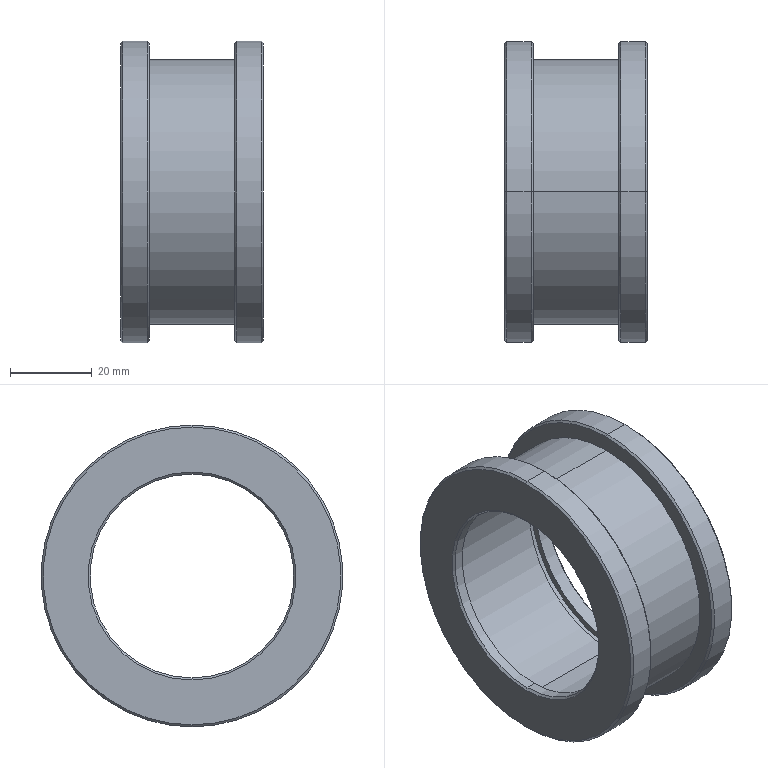Part | SolidWorks | features ICE 2, Chamfer 1, RevCut 1, Revolution 1 | 1 solid | 33 faces | box 35 x 74 x 74 mm | volume 47236 mm3 | cylinder 14 | cone 12 | plane 7 | commonest cylinder face diameters 55 x4 74 x4 50 x2 58 x2 65 x2
STEP:
#1=CARTESIAN_POINT('',(13.5,0.,-29.));
#2=VERTEX_POINT('',#1);
#3=CARTESIAN_POINT('',(13.5,0.,29.));
#4=VERTEX_POINT('',#3);
#5=CARTESIAN_POINT('',(13.5,0.,0.));
#6=DIRECTION('',(-1.,0.,0.));
#7=DIRECTION('',(0.,0.,1.));
#8=AXIS2_PLACEMENT_3D('',#5,#6,#7);
#9=CIRCLE('',#8,29.);
#10=EDGE_CURVE('',#2,#4,#9,.T.);
#11=ORIENTED_EDGE('',*,*,#10,.F.);
#12=CARTESIAN_POINT('',(11.3,0.,-29.));
#13=VERTEX_POINT('',#12);
#14=CARTESIAN_POINT('',(0.,0.,-29.));
#15=DIRECTION('',(-1.,0.,0.));
#16=VECTOR('',#15,1000.);
#17=LINE('',#14,#16);
#18=EDGE_CURVE('',#2,#13,#17,.T.);
#19=ORIENTED_EDGE('',*,*,#18,.T.);
#20=CARTESIAN_POINT('',(11.3,0.,29.));
#21=VERTEX_POINT('',#20);
#22=CARTESIAN_POINT('',(11.3,0.,0.));
#23=DIRECTION('',(-1.,0.,0.));
#24=DIRECTION('',(0.,0.,1.));
#25=AXIS2_PLACEMENT_3D('',#22,#23,#24);
#26=CIRCLE('',#25,29.);
#27=EDGE_CURVE('',#13,#21,#26,.T.);
#28=ORIENTED_EDGE('',*,*,#27,.T.);
#29=CARTESIAN_POINT('',(0.,0.,29.));
#30=DIRECTION('',(-1.,0.,0.));
#31=VECTOR('',#30,1000.);
#32=LINE('',#29,#31);
#33=EDGE_CURVE('',#4,#21,#32,.T.);
#34=ORIENTED_EDGE('',*,*,#33,.F.);
#35=EDGE_LOOP('',(#11,#19,#28,#34));
#36=FACE_OUTER_BOUND('',#35,.T.);
#37=CARTESIAN_POINT('',(0.,0.,0.));
#38=DIRECTION('',(-1.,0.,0.));
#39=DIRECTION('',(0.,0.,1.));
#40=AXIS2_PLACEMENT_3D('',#37,#38,#39);
#41=CYLINDRICAL_SURFACE('',#40,29.);
#42=ADVANCED_FACE('',(#36),#41,.F.);
#43=CARTESIAN_POINT('',(-10.5,0.,-36.5));
#44=VERTEX_POINT('',#43);
#45=CARTESIAN_POINT('',(-10.5,0.,36.5));
#46=VERTEX_POINT('',#45);
#47=CARTESIAN_POINT('',(-10.5,0.,0.));
#48=DIRECTION('',(1.,0.,0.));
#49=DIRECTION('',(0.,0.,1.));
#50=AXIS2_PLACEMENT_3D('',#47,#48,#49);
#51=CIRCLE('',#50,36.5);
#52=EDGE_CURVE('',#44,#46,#51,.T.);
#53=ORIENTED_EDGE('',*,*,#52,.F.);
#54=CARTESIAN_POINT('',(-11.,0.,-37.));
#55=VERTEX_POINT('',#54);
#56=CARTESIAN_POINT('',(-11.,0.,-37.));
#57=DIRECTION('',(-0.7071,0.,-0.7071));
#58=VECTOR('',#57,1000.);
#59=LINE('',#56,#58);
#60=EDGE_CURVE('',#44,#55,#59,.T.);
#61=ORIENTED_EDGE('',*,*,#60,.T.);
#62=CARTESIAN_POINT('',(-11.,0.,37.));
#63=VERTEX_POINT('',#62);
#64=CARTESIAN_POINT('',(-11.,0.,0.));
#65=DIRECTION('',(-1.,0.,0.));
#66=DIRECTION('',(0.,0.,1.));
#67=AXIS2_PLACEMENT_3D('',#64,#65,#66);
#68=CIRCLE('',#67,37.);
#69=EDGE_CURVE('',#63,#55,#68,.T.);
#70=ORIENTED_EDGE('',*,*,#69,.F.);
#71=CARTESIAN_POINT('',(-11.,0.,37.));
#72=DIRECTION('',(-0.7071,0.,0.7071));
#73=VECTOR('',#72,1000.);
#74=LINE('',#71,#73);
#75=EDGE_CURVE('',#46,#63,#74,.T.);
#76=ORIENTED_EDGE('',*,*,#75,.F.);
#77=EDGE_LOOP('',(#53,#61,#70,#76));
#78=FACE_OUTER_BOUND('',#77,.T.);
#79=CARTESIAN_POINT('',(-11.,0.,0.));
#80=DIRECTION('',(-1.,0.,0.));
#81=DIRECTION('',(0.,0.,1.));
#82=AXIS2_PLACEMENT_3D('',#79,#80,#81);
#83=CONICAL_SURFACE('',#82,37.,0.7854);
#84=ADVANCED_FACE('',(#78),#83,.T.);
#85=CARTESIAN_POINT('',(10.5,0.,36.5));
#86=VERTEX_POINT('',#85);
#87=CARTESIAN_POINT('',(10.5,0.,-36.5));
#88=VERTEX_POINT('',#87);
#89=CARTESIAN_POINT('',(10.5,0.,0.));
#90=DIRECTION('',(-1.,0.,0.));
#91=DIRECTION('',(0.,0.,-1.));
#92=AXIS2_PLACEMENT_3D('',#89,#90,#91);
#93=CIRCLE('',#92,36.5);
#94=EDGE_CURVE('',#86,#88,#93,.T.);
#95=ORIENTED_EDGE('',*,*,#94,.F.);
#96=CARTESIAN_POINT('',(11.,0.,37.));
#97=VERTEX_POINT('',#96);
#98=CARTESIAN_POINT('',(10.5,0.,36.5));
#99=DIRECTION('',(0.7071,0.,0.7071));
#100=VECTOR('',#99,1000.);
#101=LINE('',#98,#100);
#102=EDGE_CURVE('',#86,#97,#101,.T.);
#103=ORIENTED_EDGE('',*,*,#102,.T.);
#104=CARTESIAN_POINT('',(11.,0.,-37.));
#105=VERTEX_POINT('',#104);
#106=CARTESIAN_POINT('',(11.,0.,0.));
#107=DIRECTION('',(1.,0.,0.));
#108=DIRECTION('',(0.,0.,-1.));
#109=AXIS2_PLACEMENT_3D('',#106,#107,#108);
#110=CIRCLE('',#109,37.);
#111=EDGE_CURVE('',#105,#97,#110,.T.);
#112=ORIENTED_EDGE('',*,*,#111,.F.);
#113=CARTESIAN_POINT('',(10.5,0.,-36.5));
#114=DIRECTION('',(0.7071,0.,-0.7071));
#115=VECTOR('',#114,1000.);
#116=LINE('',#113,#115);
#117=EDGE_CURVE('',#88,#105,#116,.T.);
#118=ORIENTED_EDGE('',*,*,#117,.F.);
#119=EDGE_LOOP('',(#95,#103,#112,#118));
#120=FACE_OUTER_BOUND('',#119,.T.);
#121=CARTESIAN_POINT('',(10.5,0.,0.));
#122=DIRECTION('',(1.,0.,0.));
#123=DIRECTION('',(0.,0.,-1.));
#124=AXIS2_PLACEMENT_3D('',#121,#122,#123);
#125=CONICAL_SURFACE('',#124,36.5,0.7854);
#126=ADVANCED_FACE('',(#120),#125,.T.);
#127=CARTESIAN_POINT('',(17.5,0.,-36.5));
#128=VERTEX_POINT('',#127);
#129=CARTESIAN_POINT('',(17.5,0.,36.5));
#130=VERTEX_POINT('',#129);
#131=CARTESIAN_POINT('',(17.5,0.,0.));
#132=DIRECTION('',(1.,0.,0.));
#133=DIRECTION('',(0.,0.,1.));
#134=AXIS2_PLACEMENT_3D('',#131,#132,#133);
#135=CIRCLE('',#134,36.5);
#136=EDGE_CURVE('',#128,#130,#135,.T.);
#137=ORIENTED_EDGE('',*,*,#136,.F.);
#138=CARTESIAN_POINT('',(17.,0.,-37.));
#139=VERTEX_POINT('',#138);
#140=CARTESIAN_POINT('',(17.,0.,-37.));
#141=DIRECTION('',(-0.7071,0.,-0.7071));
#142=VECTOR('',#141,1000.);
#143=LINE('',#140,#142);
#144=EDGE_CURVE('',#128,#139,#143,.T.);
#145=ORIENTED_EDGE('',*,*,#144,.T.);
#146=CARTESIAN_POINT('',(17.,0.,37.));
#147=VERTEX_POINT('',#146);
#148=CARTESIAN_POINT('',(17.,0.,0.));
#149=DIRECTION('',(-1.,0.,0.));
#150=DIRECTION('',(0.,0.,1.));
#151=AXIS2_PLACEMENT_3D('',#148,#149,#150);
#152=CIRCLE('',#151,37.);
#153=EDGE_CURVE('',#147,#139,#152,.T.);
#154=ORIENTED_EDGE('',*,*,#153,.F.);
#155=CARTESIAN_POINT('',(17.,0.,37.));
#156=DIRECTION('',(-0.7071,0.,0.7071));
#157=VECTOR('',#156,1000.);
#158=LINE('',#155,#157);
#159=EDGE_CURVE('',#130,#147,#158,.T.);
#160=ORIENTED_EDGE('',*,*,#159,.F.);
#161=EDGE_LOOP('',(#137,#145,#154,#160));
#162=FACE_OUTER_BOUND('',#161,.T.);
#163=CARTESIAN_POINT('',(17.,0.,0.));
#164=DIRECTION('',(-1.,0.,0.));
#165=DIRECTION('',(0.,0.,1.));
#166=AXIS2_PLACEMENT_3D('',#163,#164,#165);
#167=CONICAL_SURFACE('',#166,37.,0.7854);
#168=ADVANCED_FACE('',(#162),#167,.T.);
#169=CARTESIAN_POINT('',(-17.5,0.,36.5));
#170=VERTEX_POINT('',#169);
#171=CARTESIAN_POINT('',(-17.5,0.,-36.5));
#172=VERTEX_POINT('',#171);
#173=CARTESIAN_POINT('',(-17.5,0.,0.));
#174=DIRECTION('',(-1.,0.,0.));
#175=DIRECTION('',(0.,0.,-1.));
#176=AXIS2_PLACEMENT_3D('',#173,#174,#175);
#177=CIRCLE('',#176,36.5);
#178=EDGE_CURVE('',#170,#172,#177,.T.);
#179=ORIENTED_EDGE('',*,*,#178,.F.);
#180=CARTESIAN_POINT('',(-17.,0.,37.));
#181=VERTEX_POINT('',#180);
#182=CARTESIAN_POINT('',(-17.5,0.,36.5));
#183=DIRECTION('',(0.7071,0.,0.7071));
#184=VECTOR('',#183,1000.);
#185=LINE('',#182,#184);
#186=EDGE_CURVE('',#170,#181,#185,.T.);
#187=ORIENTED_EDGE('',*,*,#186,.T.);
#188=CARTESIAN_POINT('',(-17.,0.,-37.));
#189=VERTEX_POINT('',#188);
#190=CARTESIAN_POINT('',(-17.,0.,0.));
#191=DIRECTION('',(1.,0.,0.));
#192=DIRECTION('',(0.,0.,-1.));
#193=AXIS2_PLACEMENT_3D('',#190,#191,#192);
#194=CIRCLE('',#193,37.);
#195=EDGE_CURVE('',#189,#181,#194,.T.);
#196=ORIENTED_EDGE('',*,*,#195,.F.);
#197=CARTESIAN_POINT('',(-17.5,0.,-36.5));
#198=DIRECTION('',(0.7071,0.,-0.7071));
#199=VECTOR('',#198,1000.);
#200=LINE('',#197,#199);
#201=EDGE_CURVE('',#172,#189,#200,.T.);
#202=ORIENTED_EDGE('',*,*,#201,.F.);
#203=EDGE_LOOP('',(#179,#187,#196,#202));
#204=FACE_OUTER_BOUND('',#203,.T.);
#205=CARTESIAN_POINT('',(-17.5,0.,0.));
#206=DIRECTION('',(1.,0.,0.));
#207=DIRECTION('',(0.,0.,-1.));
#208=AXIS2_PLACEMENT_3D('',#205,#206,#207);
#209=CONICAL_SURFACE('',#208,36.5,0.7854);
#210=ADVANCED_FACE('',(#204),#209,.T.);
#211=CARTESIAN_POINT('',(17.,0.,27.5));
#212=VERTEX_POINT('',#211);
#213=CARTESIAN_POINT('',(17.,0.,-27.5));
#214=VERTEX_POINT('',#213);
#215=CARTESIAN_POINT('',(17.,0.,0.));
#216=DIRECTION('',(1.,0.,0.));
#217=DIRECTION('',(0.,0.,1.));
#218=AXIS2_PLACEMENT_3D('',#215,#216,#217);
#219=CIRCLE('',#218,27.5);
#220=EDGE_CURVE('',#212,#214,#219,.T.);
#221=ORIENTED_EDGE('',*,*,#220,.F.);
#222=CARTESIAN_POINT('',(17.5,0.,28.));
#223=VERTEX_POINT('',#222);
#224=CARTESIAN_POINT('',(17.,0.,27.5));
#225=DIRECTION('',(0.7071,0.,0.7071));
#226=VECTOR('',#225,1000.);
#227=LINE('',#224,#226);
#228=EDGE_CURVE('',#212,#223,#227,.T.);
#229=ORIENTED_EDGE('',*,*,#228,.T.);
#230=CARTESIAN_POINT('',(17.5,0.,-28.));
#231=VERTEX_POINT('',#230);
#232=CARTESIAN_POINT('',(17.5,0.,0.));
#233=DIRECTION('',(-1.,0.,0.));
#234=DIRECTION('',(0.,0.,1.));
#235=AXIS2_PLACEMENT_3D('',#232,#233,#234);
#236=CIRCLE('',#235,28.);
#237=EDGE_CURVE('',#231,#223,#236,.T.);
#238=ORIENTED_EDGE('',*,*,#237,.F.);
#239=CARTESIAN_POINT('',(17.,0.,-27.5));
#240=DIRECTION('',(0.7071,0.,-0.7071));
#241=VECTOR('',#240,1000.);
#242=LINE('',#239,#241);
#243=EDGE_CURVE('',#214,#231,#242,.T.);
#244=ORIENTED_EDGE('',*,*,#243,.F.);
#245=EDGE_LOOP('',(#221,#229,#238,#244));
#246=FACE_OUTER_BOUND('',#245,.T.);
#247=CARTESIAN_POINT('',(17.,0.,0.));
#248=DIRECTION('',(1.,0.,0.));
#249=DIRECTION('',(0.,0.,-1.));
#250=AXIS2_PLACEMENT_3D('',#247,#248,#249);
#251=CONICAL_SURFACE('',#250,27.5,0.7854);
#252=ADVANCED_FACE('',(#246),#251,.F.);
#253=CARTESIAN_POINT('',(-17.,0.,-25.));
#254=VERTEX_POINT('',#253);
#255=CARTESIAN_POINT('',(-17.,0.,25.));
#256=VERTEX_POINT('',#255);
#257=CARTESIAN_POINT('',(-17.,0.,0.));
#258=DIRECTION('',(-1.,0.,0.));
#259=DIRECTION('',(0.,0.,-1.));
#260=AXIS2_PLACEMENT_3D('',#257,#258,#259);
#261=CIRCLE('',#260,25.);
#262=EDGE_CURVE('',#254,#256,#261,.T.);
#263=ORIENTED_EDGE('',*,*,#262,.F.);
#264=CARTESIAN_POINT('',(-17.5,0.,-25.5));
#265=VERTEX_POINT('',#264);
#266=CARTESIAN_POINT('',(-17.5,0.,-25.5));
#267=DIRECTION('',(-0.7071,0.,-0.7071));
#268=VECTOR('',#267,1000.);
#269=LINE('',#266,#268);
#270=EDGE_CURVE('',#254,#265,#269,.T.);
#271=ORIENTED_EDGE('',*,*,#270,.T.);
#272=CARTESIAN_POINT('',(-17.5,0.,25.5));
#273=VERTEX_POINT('',#272);
#274=CARTESIAN_POINT('',(-17.5,0.,0.));
#275=DIRECTION('',(1.,0.,0.));
#276=DIRECTION('',(0.,0.,-1.));
#277=AXIS2_PLACEMENT_3D('',#274,#275,#276);
#278=CIRCLE('',#277,25.5);
#279=EDGE_CURVE('',#273,#265,#278,.T.);
#280=ORIENTED_EDGE('',*,*,#279,.F.);
#281=CARTESIAN_POINT('',(-17.5,0.,25.5));
#282=DIRECTION('',(-0.7071,0.,0.7071));
#283=VECTOR('',#282,1000.);
#284=LINE('',#281,#283);
#285=EDGE_CURVE('',#256,#273,#284,.T.);
#286=ORIENTED_EDGE('',*,*,#285,.F.);
#287=EDGE_LOOP('',(#263,#271,#280,#286));
#288=FACE_OUTER_BOUND('',#287,.T.);
#289=CARTESIAN_POINT('',(-17.5,0.,0.));
#290=DIRECTION('',(-1.,0.,0.));
#291=DIRECTION('',(0.,0.,1.));
#292=AXIS2_PLACEMENT_3D('',#289,#290,#291);
#293=CONICAL_SURFACE('',#292,25.5,0.7854);
#294=ADVANCED_FACE('',(#288),#293,.F.);
#295=ORIENTED_EDGE('',*,*,#262,.T.);
#296=CARTESIAN_POINT('',(-14.5,0.,25.));
#297=VERTEX_POINT('',#296);
#298=CARTESIAN_POINT('',(-44.5,0.,25.));
#299=DIRECTION('',(1.,0.,0.));
#300=VECTOR('',#299,1000.);
#301=LINE('',#298,#300);
#302=EDGE_CURVE('',#256,#297,#301,.T.);
#303=ORIENTED_EDGE('',*,*,#302,.T.);
#304=CARTESIAN_POINT('',(-14.5,0.,-25.));
#305=VERTEX_POINT('',#304);
#306=CARTESIAN_POINT('',(-14.5,0.,0.));
#307=DIRECTION('',(1.,0.,0.));
#308=DIRECTION('',(0.,0.,-1.));
#309=AXIS2_PLACEMENT_3D('',#306,#307,#308);
#310=CIRCLE('',#309,25.);
#311=EDGE_CURVE('',#297,#305,#310,.T.);
#312=ORIENTED_EDGE('',*,*,#311,.T.);
#313=CARTESIAN_POINT('',(-44.5,0.,-25.));
#314=DIRECTION('',(1.,0.,0.));
#315=VECTOR('',#314,1000.);
#316=LINE('',#313,#315);
#317=EDGE_CURVE('',#254,#305,#316,.T.);
#318=ORIENTED_EDGE('',*,*,#317,.F.);
#319=EDGE_LOOP('',(#295,#303,#312,#318));
#320=FACE_OUTER_BOUND('',#319,.T.);
#321=CARTESIAN_POINT('',(-44.5,0.,0.));
#322=DIRECTION('',(1.,0.,0.));
#323=DIRECTION('',(0.,0.,-1.));
#324=AXIS2_PLACEMENT_3D('',#321,#322,#323);
#325=CYLINDRICAL_SURFACE('',#324,25.);
#326=ADVANCED_FACE('',(#320),#325,.F.);
#327=ORIENTED_EDGE('',*,*,#69,.T.);
#328=CARTESIAN_POINT('',(-17.5,0.,-37.));
#329=DIRECTION('',(-1.,0.,0.));
#330=VECTOR('',#329,1000.);
#331=LINE('',#328,#330);
#332=EDGE_CURVE('',#55,#189,#331,.T.);
#333=ORIENTED_EDGE('',*,*,#332,.T.);
#334=ORIENTED_EDGE('',*,*,#195,.T.);
#335=CARTESIAN_POINT('',(-17.5,0.,37.));
#336=DIRECTION('',(-1.,0.,0.));
#337=VECTOR('',#336,1000.);
#338=LINE('',#335,#337);
#339=EDGE_CURVE('',#63,#181,#338,.T.);
#340=ORIENTED_EDGE('',*,*,#339,.F.);
#341=EDGE_LOOP('',(#327,#333,#334,#340));
#342=FACE_OUTER_BOUND('',#341,.T.);
#343=CARTESIAN_POINT('',(-17.5,0.,0.));
#344=DIRECTION('',(-1.,0.,0.));
#345=DIRECTION('',(0.,0.,1.));
#346=AXIS2_PLACEMENT_3D('',#343,#344,#345);
#347=CYLINDRICAL_SURFACE('',#346,37.);
#348=ADVANCED_FACE('',(#342),#347,.T.);
#349=CARTESIAN_POINT('',(10.5,0.,32.5));
#350=VERTEX_POINT('',#349);
#351=CARTESIAN_POINT('',(10.5,0.,-32.5));
#352=VERTEX_POINT('',#351);
#353=CARTESIAN_POINT('',(10.5,0.,0.));
#354=DIRECTION('',(-1.,0.,0.));
#355=DIRECTION('',(0.,0.,1.));
#356=AXIS2_PLACEMENT_3D('',#353,#354,#355);
#357=CIRCLE('',#356,32.5);
#358=EDGE_CURVE('',#350,#352,#357,.T.);
#359=ORIENTED_EDGE('',*,*,#358,.T.);
#360=CARTESIAN_POINT('',(-10.5,0.,-32.5));
#361=VERTEX_POINT('',#360);
#362=CARTESIAN_POINT('',(-17.5,0.,-32.5));
#363=DIRECTION('',(-1.,0.,0.));
#364=VECTOR('',#363,1000.);
#365=LINE('',#362,#364);
#366=EDGE_CURVE('',#352,#361,#365,.T.);
#367=ORIENTED_EDGE('',*,*,#366,.T.);
#368=CARTESIAN_POINT('',(-10.5,0.,32.5));
#369=VERTEX_POINT('',#368);
#370=CARTESIAN_POINT('',(-10.5,0.,0.));
#371=DIRECTION('',(-1.,0.,0.));
#372=DIRECTION('',(0.,0.,1.));
#373=AXIS2_PLACEMENT_3D('',#370,#371,#372);
#374=CIRCLE('',#373,32.5);
#375=EDGE_CURVE('',#369,#361,#374,.T.);
#376=ORIENTED_EDGE('',*,*,#375,.F.);
#377=CARTESIAN_POINT('',(-17.5,0.,32.5));
#378=DIRECTION('',(-1.,0.,0.));
#379=VECTOR('',#378,1000.);
#380=LINE('',#377,#379);
#381=EDGE_CURVE('',#350,#369,#380,.T.);
#382=ORIENTED_EDGE('',*,*,#381,.F.);
#383=EDGE_LOOP('',(#359,#367,#376,#382));
#384=FACE_OUTER_BOUND('',#383,.T.);
#385=CARTESIAN_POINT('',(-17.5,0.,0.));
#386=DIRECTION('',(-1.,0.,0.));
#387=DIRECTION('',(0.,0.,1.));
#388=AXIS2_PLACEMENT_3D('',#385,#386,#387);
#389=CYLINDRICAL_SURFACE('',#388,32.5);
#390=ADVANCED_FACE('',(#384),#389,.T.);
#391=ORIENTED_EDGE('',*,*,#153,.T.);
#392=CARTESIAN_POINT('',(-17.5,0.,-37.));
#393=DIRECTION('',(-1.,0.,0.));
#394=VECTOR('',#393,1000.);
#395=LINE('',#392,#394);
#396=EDGE_CURVE('',#139,#105,#395,.T.);
#397=ORIENTED_EDGE('',*,*,#396,.T.);
#398=ORIENTED_EDGE('',*,*,#111,.T.);
#399=CARTESIAN_POINT('',(-17.5,0.,37.));
#400=DIRECTION('',(-1.,0.,0.));
#401=VECTOR('',#400,1000.);
#402=LINE('',#399,#401);
#403=EDGE_CURVE('',#147,#97,#402,.T.);
#404=ORIENTED_EDGE('',*,*,#403,.F.);
#405=EDGE_LOOP('',(#391,#397,#398,#404));
#406=FACE_OUTER_BOUND('',#405,.T.);
#407=CARTESIAN_POINT('',(-17.5,0.,0.));
#408=DIRECTION('',(-1.,0.,0.));
#409=DIRECTION('',(0.,0.,1.));
#410=AXIS2_PLACEMENT_3D('',#407,#408,#409);
#411=CYLINDRICAL_SURFACE('',#410,37.);
#412=ADVANCED_FACE('',(#406),#411,.T.);
#413=CARTESIAN_POINT('',(13.5,0.,-27.5));
#414=VERTEX_POINT('',#413);
#415=CARTESIAN_POINT('',(13.5,0.,27.5));
#416=VERTEX_POINT('',#415);
#417=CARTESIAN_POINT('',(13.5,0.,0.));
#418=DIRECTION('',(-1.,0.,0.));
#419=DIRECTION('',(0.,0.,1.));
#420=AXIS2_PLACEMENT_3D('',#417,#418,#419);
#421=CIRCLE('',#420,27.5);
#422=EDGE_CURVE('',#414,#416,#421,.T.);
#423=ORIENTED_EDGE('',*,*,#422,.T.);
#424=CARTESIAN_POINT('',(-14.5,0.,27.5));
#425=DIRECTION('',(1.,0.,0.));
#426=VECTOR('',#425,1000.);
#427=LINE('',#424,#426);
#428=EDGE_CURVE('',#416,#212,#427,.T.);
#429=ORIENTED_EDGE('',*,*,#428,.T.);
#430=ORIENTED_EDGE('',*,*,#220,.T.);
#431=CARTESIAN_POINT('',(-14.5,0.,-27.5));
#432=DIRECTION('',(1.,0.,0.));
#433=VECTOR('',#432,1000.);
#434=LINE('',#431,#433);
#435=EDGE_CURVE('',#414,#214,#434,.T.);
#436=ORIENTED_EDGE('',*,*,#435,.F.);
#437=EDGE_LOOP('',(#423,#429,#430,#436));
#438=FACE_OUTER_BOUND('',#437,.T.);
#439=CARTESIAN_POINT('',(-14.5,0.,0.));
#440=DIRECTION('',(1.,0.,0.));
#441=DIRECTION('',(0.,0.,-1.));
#442=AXIS2_PLACEMENT_3D('',#439,#440,#441);
#443=CYLINDRICAL_SURFACE('',#442,27.5);
#444=ADVANCED_FACE('',(#438),#443,.F.);
#445=CARTESIAN_POINT('',(-14.5,0.,27.5));
#446=VERTEX_POINT('',#445);
#447=CARTESIAN_POINT('',(-14.5,0.,-27.5));
#448=VERTEX_POINT('',#447);
#449=CARTESIAN_POINT('',(-14.5,0.,0.));
#450=DIRECTION('',(1.,0.,0.));
#451=DIRECTION('',(0.,0.,-1.));
#452=AXIS2_PLACEMENT_3D('',#449,#450,#451);
#453=CIRCLE('',#452,27.5);
#454=EDGE_CURVE('',#446,#448,#453,.T.);
#455=ORIENTED_EDGE('',*,*,#454,.F.);
#456=CARTESIAN_POINT('',(11.3,0.,27.5));
#457=VERTEX_POINT('',#456);
#458=CARTESIAN_POINT('',(-14.5,0.,27.5));
#459=DIRECTION('',(1.,0.,0.));
#460=VECTOR('',#459,1000.);
#461=LINE('',#458,#460);
#462=EDGE_CURVE('',#446,#457,#461,.T.);
#463=ORIENTED_EDGE('',*,*,#462,.T.);
#464=CARTESIAN_POINT('',(11.3,0.,-27.5));
#465=VERTEX_POINT('',#464);
#466=CARTESIAN_POINT('',(11.3,0.,0.));
#467=DIRECTION('',(-1.,0.,0.));
#468=DIRECTION('',(0.,0.,1.));
#469=AXIS2_PLACEMENT_3D('',#466,#467,#468);
#470=CIRCLE('',#469,27.5);
#471=EDGE_CURVE('',#465,#457,#470,.T.);
#472=ORIENTED_EDGE('',*,*,#471,.F.);
#473=CARTESIAN_POINT('',(-14.5,0.,-27.5));
#474=DIRECTION('',(1.,0.,0.));
#475=VECTOR('',#474,1000.);
#476=LINE('',#473,#475);
#477=EDGE_CURVE('',#448,#465,#476,.T.);
#478=ORIENTED_EDGE('',*,*,#477,.F.);
#479=EDGE_LOOP('',(#455,#463,#472,#478));
#480=FACE_OUTER_BOUND('',#479,.T.);
#481=CARTESIAN_POINT('',(-14.5,0.,0.));
#482=DIRECTION('',(1.,0.,0.));
#483=DIRECTION('',(0.,0.,-1.));
#484=AXIS2_PLACEMENT_3D('',#481,#482,#483);
#485=CYLINDRICAL_SURFACE('',#484,27.5);
#486=ADVANCED_FACE('',(#480),#485,.F.);
#487=ORIENTED_EDGE('',*,*,#462,.F.);
#488=CARTESIAN_POINT('',(-14.5,0.,0.));
#489=DIRECTION('',(1.,0.,0.));
#490=DIRECTION('',(0.,0.,-1.));
#491=AXIS2_PLACEMENT_3D('',#488,#489,#490);
#492=CIRCLE('',#491,27.5);
#493=EDGE_CURVE('',#448,#446,#492,.T.);
#494=ORIENTED_EDGE('',*,*,#493,.F.);
#495=ORIENTED_EDGE('',*,*,#477,.T.);
#496=CARTESIAN_POINT('',(11.3,0.,0.));
#497=DIRECTION('',(-1.,0.,0.));
#498=DIRECTION('',(0.,0.,1.));
#499=AXIS2_PLACEMENT_3D('',#496,#497,#498);
#500=CIRCLE('',#499,27.5);
#501=EDGE_CURVE('',#457,#465,#500,.T.);
#502=ORIENTED_EDGE('',*,*,#501,.F.);
#503=EDGE_LOOP('',(#487,#494,#495,#502));
#504=FACE_OUTER_BOUND('',#503,.T.);
#505=CARTESIAN_POINT('',(-14.5,0.,0.));
#506=DIRECTION('',(1.,0.,0.));
#507=DIRECTION('',(0.,0.,-1.));
#508=AXIS2_PLACEMENT_3D('',#505,#506,#507);
#509=CYLINDRICAL_SURFACE('',#508,27.5);
#510=ADVANCED_FACE('',(#504),#509,.F.);
#511=ORIENTED_EDGE('',*,*,#428,.F.);
#512=CARTESIAN_POINT('',(13.5,0.,0.));
#513=DIRECTION('',(-1.,0.,0.));
#514=DIRECTION('',(0.,0.,1.));
#515=AXIS2_PLACEMENT_3D('',#512,#513,#514);
#516=CIRCLE('',#515,27.5);
#517=EDGE_CURVE('',#416,#414,#516,.T.);
#518=ORIENTED_EDGE('',*,*,#517,.T.);
#519=ORIENTED_EDGE('',*,*,#435,.T.);
#520=CARTESIAN_POINT('',(17.,0.,0.));
#521=DIRECTION('',(1.,0.,0.));
#522=DIRECTION('',(0.,0.,1.));
#523=AXIS2_PLACEMENT_3D('',#520,#521,#522);
#524=CIRCLE('',#523,27.5);
#525=EDGE_CURVE('',#214,#212,#524,.T.);
#526=ORIENTED_EDGE('',*,*,#525,.T.);
#527=EDGE_LOOP('',(#511,#518,#519,#526));
#528=FACE_OUTER_BOUND('',#527,.T.);
#529=CARTESIAN_POINT('',(-14.5,0.,0.));
#530=DIRECTION('',(1.,0.,0.));
#531=DIRECTION('',(0.,0.,-1.));
#532=AXIS2_PLACEMENT_3D('',#529,#530,#531);
#533=CYLINDRICAL_SURFACE('',#532,27.5);
#534=ADVANCED_FACE('',(#528),#533,.F.);
#535=ORIENTED_EDGE('',*,*,#279,.T.);
#536=CARTESIAN_POINT('',(-17.5,0.,0.));
#537=DIRECTION('',(1.,0.,0.));
#538=DIRECTION('',(0.,0.,-1.));
#539=AXIS2_PLACEMENT_3D('',#536,#537,#538);
#540=CIRCLE('',#539,25.5);
#541=EDGE_CURVE('',#265,#273,#540,.T.);
#542=ORIENTED_EDGE('',*,*,#541,.T.);
#543=EDGE_LOOP('',(#535,#542));
#544=FACE_BOUND('',#543,.T.);
#545=CARTESIAN_POINT('',(-17.5,0.,0.));
#546=DIRECTION('',(-1.,0.,0.));
#547=DIRECTION('',(0.,0.,-1.));
#548=AXIS2_PLACEMENT_3D('',#545,#546,#547);
#549=CIRCLE('',#548,36.5);
#550=EDGE_CURVE('',#172,#170,#549,.T.);
#551=ORIENTED_EDGE('',*,*,#550,.T.);
#552=ORIENTED_EDGE('',*,*,#178,.T.);
#553=EDGE_LOOP('',(#551,#552));
#554=FACE_OUTER_BOUND('',#553,.T.);
#555=CARTESIAN_POINT('',(-17.5,37.,0.));
#556=DIRECTION('',(1.,0.,0.));
#557=DIRECTION('',(0.,0.,-1.));
#558=AXIS2_PLACEMENT_3D('',#555,#556,#557);
#559=PLANE('',#558);
#560=ADVANCED_FACE('',(#544,#554),#559,.F.);
#561=ORIENTED_EDGE('',*,*,#237,.T.);
#562=CARTESIAN_POINT('',(17.5,0.,0.));
#563=DIRECTION('',(-1.,0.,0.));
#564=DIRECTION('',(0.,0.,1.));
#565=AXIS2_PLACEMENT_3D('',#562,#563,#564);
#566=CIRCLE('',#565,28.);
#567=EDGE_CURVE('',#223,#231,#566,.T.);
#568=ORIENTED_EDGE('',*,*,#567,.T.);
#569=EDGE_LOOP('',(#561,#568));
#570=FACE_BOUND('',#569,.T.);
#571=CARTESIAN_POINT('',(17.5,0.,0.));
#572=DIRECTION('',(1.,0.,0.));
#573=DIRECTION('',(0.,0.,1.));
#574=AXIS2_PLACEMENT_3D('',#571,#572,#573);
#575=CIRCLE('',#574,36.5);
#576=EDGE_CURVE('',#130,#128,#575,.T.);
#577=ORIENTED_EDGE('',*,*,#576,.T.);
#578=ORIENTED_EDGE('',*,*,#136,.T.);
#579=EDGE_LOOP('',(#577,#578));
#580=FACE_OUTER_BOUND('',#579,.T.);
#581=CARTESIAN_POINT('',(17.5,0.,0.));
#582=DIRECTION('',(-1.,0.,0.));
#583=DIRECTION('',(0.,0.,1.));
#584=AXIS2_PLACEMENT_3D('',#581,#582,#583);
#585=PLANE('',#584);
#586=ADVANCED_FACE('',(#570,#580),#585,.F.);
#587=ORIENTED_EDGE('',*,*,#396,.F.);
#588=CARTESIAN_POINT('',(17.,0.,0.));
#589=DIRECTION('',(-1.,0.,0.));
#590=DIRECTION('',(0.,0.,1.));
#591=AXIS2_PLACEMENT_3D('',#588,#589,#590);
#592=CIRCLE('',#591,37.);
#593=EDGE_CURVE('',#139,#147,#592,.T.);
#594=ORIENTED_EDGE('',*,*,#593,.T.);
#595=ORIENTED_EDGE('',*,*,#403,.T.);
#596=CARTESIAN_POINT('',(11.,0.,0.));
#597=DIRECTION('',(1.,0.,0.));
#598=DIRECTION('',(0.,0.,-1.));
#599=AXIS2_PLACEMENT_3D('',#596,#597,#598);
#600=CIRCLE('',#599,37.);
#601=EDGE_CURVE('',#97,#105,#600,.T.);
#602=ORIENTED_EDGE('',*,*,#601,.T.);
#603=EDGE_LOOP('',(#587,#594,#595,#602));
#604=FACE_OUTER_BOUND('',#603,.T.);
#605=CARTESIAN_POINT('',(-17.5,0.,0.));
#606=DIRECTION('',(-1.,0.,0.));
#607=DIRECTION('',(0.,0.,1.));
#608=AXIS2_PLACEMENT_3D('',#605,#606,#607);
#609=CYLINDRICAL_SURFACE('',#608,37.);
#610=ADVANCED_FACE('',(#604),#609,.T.);
#611=CARTESIAN_POINT('',(10.5,0.,0.));
#612=DIRECTION('',(-1.,0.,0.));
#613=DIRECTION('',(0.,0.,-1.));
#614=AXIS2_PLACEMENT_3D('',#611,#612,#613);
#615=CIRCLE('',#614,36.5);
#616=EDGE_CURVE('',#88,#86,#615,.T.);
#617=ORIENTED_EDGE('',*,*,#616,.T.);
#618=ORIENTED_EDGE('',*,*,#94,.T.);
#619=EDGE_LOOP('',(#617,#618));
#620=FACE_OUTER_BOUND('',#619,.T.);
#621=ORIENTED_EDGE('',*,*,#358,.F.);
#622=CARTESIAN_POINT('',(10.5,0.,0.));
#623=DIRECTION('',(-1.,0.,0.));
#624=DIRECTION('',(0.,0.,1.));
#625=AXIS2_PLACEMENT_3D('',#622,#623,#624);
#626=CIRCLE('',#625,32.5);
#627=EDGE_CURVE('',#352,#350,#626,.T.);
#628=ORIENTED_EDGE('',*,*,#627,.F.);
#629=EDGE_LOOP('',(#621,#628));
#630=FACE_BOUND('',#629,.T.);
#631=CARTESIAN_POINT('',(10.5,37.,0.));
#632=DIRECTION('',(1.,0.,0.));
#633=DIRECTION('',(0.,0.,-1.));
#634=AXIS2_PLACEMENT_3D('',#631,#632,#633);
#635=PLANE('',#634);
#636=ADVANCED_FACE('',(#620,#630),#635,.F.);
#637=ORIENTED_EDGE('',*,*,#366,.F.);
#638=ORIENTED_EDGE('',*,*,#627,.T.);
#639=ORIENTED_EDGE('',*,*,#381,.T.);
#640=CARTESIAN_POINT('',(-10.5,0.,0.));
#641=DIRECTION('',(-1.,0.,0.));
#642=DIRECTION('',(0.,0.,1.));
#643=AXIS2_PLACEMENT_3D('',#640,#641,#642);
#644=CIRCLE('',#643,32.5);
#645=EDGE_CURVE('',#361,#369,#644,.T.);
#646=ORIENTED_EDGE('',*,*,#645,.F.);
#647=EDGE_LOOP('',(#637,#638,#639,#646));
#648=FACE_OUTER_BOUND('',#647,.T.);
#649=CARTESIAN_POINT('',(-17.5,0.,0.));
#650=DIRECTION('',(-1.,0.,0.));
#651=DIRECTION('',(0.,0.,1.));
#652=AXIS2_PLACEMENT_3D('',#649,#650,#651);
#653=CYLINDRICAL_SURFACE('',#652,32.5);
#654=ADVANCED_FACE('',(#648),#653,.T.);
#655=CARTESIAN_POINT('',(-10.5,0.,0.));
#656=DIRECTION('',(1.,0.,0.));
#657=DIRECTION('',(0.,0.,1.));
#658=AXIS2_PLACEMENT_3D('',#655,#656,#657);
#659=CIRCLE('',#658,36.5);
#660=EDGE_CURVE('',#46,#44,#659,.T.);
#661=ORIENTED_EDGE('',*,*,#660,.T.);
#662=ORIENTED_EDGE('',*,*,#52,.T.);
#663=EDGE_LOOP('',(#661,#662));
#664=FACE_OUTER_BOUND('',#663,.T.);
#665=ORIENTED_EDGE('',*,*,#375,.T.);
#666=ORIENTED_EDGE('',*,*,#645,.T.);
#667=EDGE_LOOP('',(#665,#666));
#668=FACE_BOUND('',#667,.T.);
#669=CARTESIAN_POINT('',(-10.5,32.5,0.));
#670=DIRECTION('',(-1.,0.,0.));
#671=DIRECTION('',(0.,0.,1.));
#672=AXIS2_PLACEMENT_3D('',#669,#670,#671);
#673=PLANE('',#672);
#674=ADVANCED_FACE('',(#664,#668),#673,.F.);
#675=ORIENTED_EDGE('',*,*,#332,.F.);
#676=CARTESIAN_POINT('',(-11.,0.,0.));
#677=DIRECTION('',(-1.,0.,0.));
#678=DIRECTION('',(0.,0.,1.));
#679=AXIS2_PLACEMENT_3D('',#676,#677,#678);
#680=CIRCLE('',#679,37.);
#681=EDGE_CURVE('',#55,#63,#680,.T.);
#682=ORIENTED_EDGE('',*,*,#681,.T.);
#683=ORIENTED_EDGE('',*,*,#339,.T.);
#684=CARTESIAN_POINT('',(-17.,0.,0.));
#685=DIRECTION('',(1.,0.,0.));
#686=DIRECTION('',(0.,0.,-1.));
#687=AXIS2_PLACEMENT_3D('',#684,#685,#686);
#688=CIRCLE('',#687,37.);
#689=EDGE_CURVE('',#181,#189,#688,.T.);
#690=ORIENTED_EDGE('',*,*,#689,.T.);
#691=EDGE_LOOP('',(#675,#682,#683,#690));
#692=FACE_OUTER_BOUND('',#691,.T.);
#693=CARTESIAN_POINT('',(-17.5,0.,0.));
#694=DIRECTION('',(-1.,0.,0.));
#695=DIRECTION('',(0.,0.,1.));
#696=AXIS2_PLACEMENT_3D('',#693,#694,#695);
#697=CYLINDRICAL_SURFACE('',#696,37.);
#698=ADVANCED_FACE('',(#692),#697,.T.);
#699=CARTESIAN_POINT('',(-14.5,0.,0.));
#700=DIRECTION('',(1.,0.,0.));
#701=DIRECTION('',(0.,0.,-1.));
#702=AXIS2_PLACEMENT_3D('',#699,#700,#701);
#703=CIRCLE('',#702,25.);
#704=EDGE_CURVE('',#305,#297,#703,.T.);
#705=ORIENTED_EDGE('',*,*,#704,.F.);
#706=ORIENTED_EDGE('',*,*,#311,.F.);
#707=EDGE_LOOP('',(#705,#706));
#708=FACE_BOUND('',#707,.T.);
#709=ORIENTED_EDGE('',*,*,#493,.T.);
#710=ORIENTED_EDGE('',*,*,#454,.T.);
#711=EDGE_LOOP('',(#709,#710));
#712=FACE_OUTER_BOUND('',#711,.T.);
#713=CARTESIAN_POINT('',(-14.5,0.,0.));
#714=DIRECTION('',(1.,0.,0.));
#715=DIRECTION('',(0.,0.,-1.));
#716=AXIS2_PLACEMENT_3D('',#713,#714,#715);
#717=PLANE('',#716);
#718=ADVANCED_FACE('',(#708,#712),#717,.T.);
#719=ORIENTED_EDGE('',*,*,#302,.F.);
#720=CARTESIAN_POINT('',(-17.,0.,0.));
#721=DIRECTION('',(-1.,0.,0.));
#722=DIRECTION('',(0.,0.,-1.));
#723=AXIS2_PLACEMENT_3D('',#720,#721,#722);
#724=CIRCLE('',#723,25.);
#725=EDGE_CURVE('',#256,#254,#724,.T.);
#726=ORIENTED_EDGE('',*,*,#725,.T.);
#727=ORIENTED_EDGE('',*,*,#317,.T.);
#728=ORIENTED_EDGE('',*,*,#704,.T.);
#729=EDGE_LOOP('',(#719,#726,#727,#728));
#730=FACE_OUTER_BOUND('',#729,.T.);
#731=CARTESIAN_POINT('',(-44.5,0.,0.));
#732=DIRECTION('',(1.,0.,0.));
#733=DIRECTION('',(0.,0.,-1.));
#734=AXIS2_PLACEMENT_3D('',#731,#732,#733);
#735=CYLINDRICAL_SURFACE('',#734,25.);
#736=ADVANCED_FACE('',(#730),#735,.F.);
#737=ORIENTED_EDGE('',*,*,#270,.F.);
#738=ORIENTED_EDGE('',*,*,#725,.F.);
#739=ORIENTED_EDGE('',*,*,#285,.T.);
#740=ORIENTED_EDGE('',*,*,#541,.F.);
#741=EDGE_LOOP('',(#737,#738,#739,#740));
#742=FACE_OUTER_BOUND('',#741,.T.);
#743=CARTESIAN_POINT('',(-17.5,0.,0.));
#744=DIRECTION('',(-1.,0.,0.));
#745=DIRECTION('',(0.,0.,1.));
#746=AXIS2_PLACEMENT_3D('',#743,#744,#745);
#747=CONICAL_SURFACE('',#746,25.5,0.7854);
#748=ADVANCED_FACE('',(#742),#747,.F.);
#749=ORIENTED_EDGE('',*,*,#228,.F.);
#750=ORIENTED_EDGE('',*,*,#525,.F.);
#751=ORIENTED_EDGE('',*,*,#243,.T.);
#752=ORIENTED_EDGE('',*,*,#567,.F.);
#753=EDGE_LOOP('',(#749,#750,#751,#752));
#754=FACE_OUTER_BOUND('',#753,.T.);
#755=CARTESIAN_POINT('',(17.,0.,0.));
#756=DIRECTION('',(1.,0.,0.));
#757=DIRECTION('',(0.,0.,-1.));
#758=AXIS2_PLACEMENT_3D('',#755,#756,#757);
#759=CONICAL_SURFACE('',#758,27.5,0.7854);
#760=ADVANCED_FACE('',(#754),#759,.F.);
#761=ORIENTED_EDGE('',*,*,#186,.F.);
#762=ORIENTED_EDGE('',*,*,#550,.F.);
#763=ORIENTED_EDGE('',*,*,#201,.T.);
#764=ORIENTED_EDGE('',*,*,#689,.F.);
#765=EDGE_LOOP('',(#761,#762,#763,#764));
#766=FACE_OUTER_BOUND('',#765,.T.);
#767=CARTESIAN_POINT('',(-17.5,0.,0.));
#768=DIRECTION('',(1.,0.,0.));
#769=DIRECTION('',(0.,0.,-1.));
#770=AXIS2_PLACEMENT_3D('',#767,#768,#769);
#771=CONICAL_SURFACE('',#770,36.5,0.7854);
#772=ADVANCED_FACE('',(#766),#771,.T.);
#773=ORIENTED_EDGE('',*,*,#144,.F.);
#774=ORIENTED_EDGE('',*,*,#576,.F.);
#775=ORIENTED_EDGE('',*,*,#159,.T.);
#776=ORIENTED_EDGE('',*,*,#593,.F.);
#777=EDGE_LOOP('',(#773,#774,#775,#776));
#778=FACE_OUTER_BOUND('',#777,.T.);
#779=CARTESIAN_POINT('',(17.,0.,0.));
#780=DIRECTION('',(-1.,0.,0.));
#781=DIRECTION('',(0.,0.,1.));
#782=AXIS2_PLACEMENT_3D('',#779,#780,#781);
#783=CONICAL_SURFACE('',#782,37.,0.7854);
#784=ADVANCED_FACE('',(#778),#783,.T.);
#785=ORIENTED_EDGE('',*,*,#102,.F.);
#786=ORIENTED_EDGE('',*,*,#616,.F.);
#787=ORIENTED_EDGE('',*,*,#117,.T.);
#788=ORIENTED_EDGE('',*,*,#601,.F.);
#789=EDGE_LOOP('',(#785,#786,#787,#788));
#790=FACE_OUTER_BOUND('',#789,.T.);
#791=CARTESIAN_POINT('',(10.5,0.,0.));
#792=DIRECTION('',(1.,0.,0.));
#793=DIRECTION('',(0.,0.,-1.));
#794=AXIS2_PLACEMENT_3D('',#791,#792,#793);
#795=CONICAL_SURFACE('',#794,36.5,0.7854);
#796=ADVANCED_FACE('',(#790),#795,.T.);
#797=ORIENTED_EDGE('',*,*,#60,.F.);
#798=ORIENTED_EDGE('',*,*,#660,.F.);
#799=ORIENTED_EDGE('',*,*,#75,.T.);
#800=ORIENTED_EDGE('',*,*,#681,.F.);
#801=EDGE_LOOP('',(#797,#798,#799,#800));
#802=FACE_OUTER_BOUND('',#801,.T.);
#803=CARTESIAN_POINT('',(-11.,0.,0.));
#804=DIRECTION('',(-1.,0.,0.));
#805=DIRECTION('',(0.,0.,1.));
#806=AXIS2_PLACEMENT_3D('',#803,#804,#805);
#807=CONICAL_SURFACE('',#806,37.,0.7854);
#808=ADVANCED_FACE('',(#802),#807,.T.);
#809=ORIENTED_EDGE('',*,*,#471,.T.);
#810=ORIENTED_EDGE('',*,*,#501,.T.);
#811=EDGE_LOOP('',(#809,#810));
#812=FACE_BOUND('',#811,.T.);
#813=CARTESIAN_POINT('',(11.3,0.,0.));
#814=DIRECTION('',(-1.,0.,0.));
#815=DIRECTION('',(0.,0.,1.));
#816=AXIS2_PLACEMENT_3D('',#813,#814,#815);
#817=CIRCLE('',#816,29.);
#818=EDGE_CURVE('',#21,#13,#817,.T.);
#819=ORIENTED_EDGE('',*,*,#818,.F.);
#820=ORIENTED_EDGE('',*,*,#27,.F.);
#821=EDGE_LOOP('',(#819,#820));
#822=FACE_OUTER_BOUND('',#821,.T.);
#823=CARTESIAN_POINT('',(11.3,0.,-27.5));
#824=DIRECTION('',(1.,0.,0.));
#825=DIRECTION('',(0.,0.,-1.));
#826=AXIS2_PLACEMENT_3D('',#823,#824,#825);
#827=PLANE('',#826);
#828=ADVANCED_FACE('',(#812,#822),#827,.T.);
#829=ORIENTED_EDGE('',*,*,#18,.F.);
#830=CARTESIAN_POINT('',(13.5,0.,0.));
#831=DIRECTION('',(-1.,0.,0.));
#832=DIRECTION('',(0.,0.,1.));
#833=AXIS2_PLACEMENT_3D('',#830,#831,#832);
#834=CIRCLE('',#833,29.);
#835=EDGE_CURVE('',#4,#2,#834,.T.);
#836=ORIENTED_EDGE('',*,*,#835,.F.);
#837=ORIENTED_EDGE('',*,*,#33,.T.);
#838=ORIENTED_EDGE('',*,*,#818,.T.);
#839=EDGE_LOOP('',(#829,#836,#837,#838));
#840=FACE_OUTER_BOUND('',#839,.T.);
#841=CARTESIAN_POINT('',(0.,0.,0.));
#842=DIRECTION('',(-1.,0.,0.));
#843=DIRECTION('',(0.,0.,1.));
#844=AXIS2_PLACEMENT_3D('',#841,#842,#843);
#845=CYLINDRICAL_SURFACE('',#844,29.);
#846=ADVANCED_FACE('',(#840),#845,.F.);
#847=ORIENTED_EDGE('',*,*,#835,.T.);
#848=ORIENTED_EDGE('',*,*,#10,.T.);
#849=EDGE_LOOP('',(#847,#848));
#850=FACE_OUTER_BOUND('',#849,.T.);
#851=ORIENTED_EDGE('',*,*,#422,.F.);
#852=ORIENTED_EDGE('',*,*,#517,.F.);
#853=EDGE_LOOP('',(#851,#852));
#854=FACE_BOUND('',#853,.T.);
#855=CARTESIAN_POINT('',(13.5,0.,-27.5));
#856=DIRECTION('',(-1.,0.,0.));
#857=DIRECTION('',(0.,0.,1.));
#858=AXIS2_PLACEMENT_3D('',#855,#856,#857);
#859=PLANE('',#858);
#860=ADVANCED_FACE('',(#850,#854),#859,.T.);
#861=CLOSED_SHELL('',(#42,#84,#126,#168,#210,#252,#294,#326,#348,#390,#412,#444,#486,#510,#534,#560,#586,#610,#636,#654,#674,#698,#718,#736,#748,#760,#772,#784,#796,#808,#828,#846,#860));
#862=MANIFOLD_SOLID_BREP('',#861);
#863=CARTESIAN_POINT('',(0.,0.,0.));
#864=DIRECTION('',(0.,0.,1.));
#865=DIRECTION('',(1.,0.,0.));
#866=AXIS2_PLACEMENT_3D('',#863,#864,#865);
#867=(LENGTH_UNIT()NAMED_UNIT(*)SI_UNIT(.MILLI.,.METRE.));
#868=UNCERTAINTY_MEASURE_WITH_UNIT(LENGTH_MEASURE(0.00001),#867,'','');
#869=(NAMED_UNIT(*)PLANE_ANGLE_UNIT()SI_UNIT($,.RADIAN.));
#870=(NAMED_UNIT(*)SI_UNIT($,.STERADIAN.)SOLID_ANGLE_UNIT());
#871=(GEOMETRIC_REPRESENTATION_CONTEXT(3)GLOBAL_UNCERTAINTY_ASSIGNED_CONTEXT((#868))GLOBAL_UNIT_ASSIGNED_CONTEXT((#867,#869,#870))REPRESENTATION_CONTEXT('',''));
#872=ADVANCED_BREP_SHAPE_REPRESENTATION('',(#862,#866),#871);